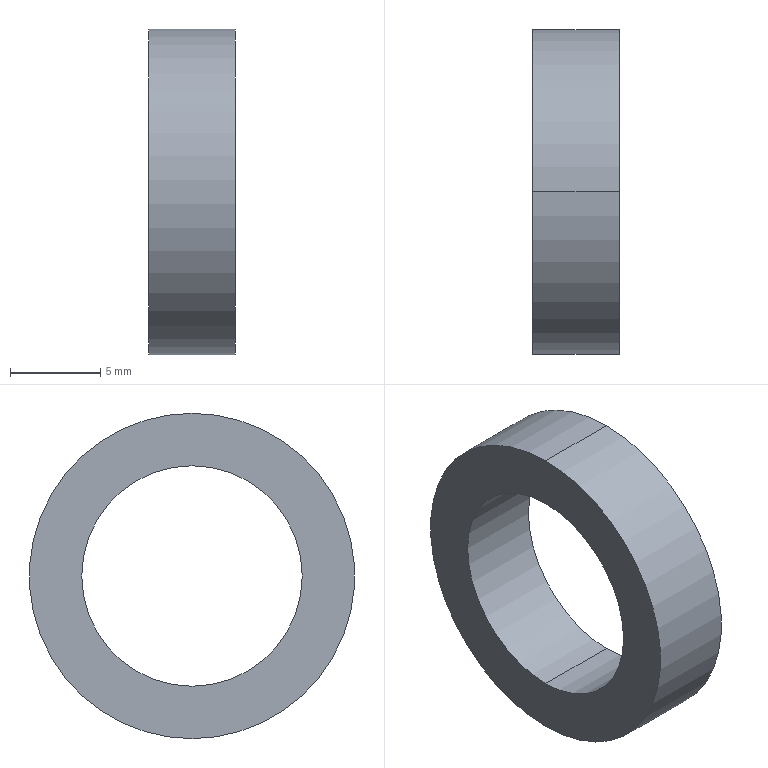Part | STEP file | Symmetry REAR WASHER BALANCER | 1 solid | 6 faces | box 4.76 x 18 x 18 mm | volume 654.835 mm3 | cylinder 4 | plane 2 | commonest cylinder face diameters 12.2 x2 18 x2
STEP:
#1=CARTESIAN_POINT('',(4.76,0.,6.1));
#2=VERTEX_POINT('',#1);
#3=CARTESIAN_POINT('',(4.76,0.,-6.1));
#4=VERTEX_POINT('',#3);
#5=CARTESIAN_POINT('',(4.76,0.,0.));
#6=DIRECTION('',(-1.,0.,0.));
#7=DIRECTION('',(0.,0.,1.));
#8=AXIS2_PLACEMENT_3D('',#5,#6,#7);
#9=CIRCLE('',#8,6.1);
#10=EDGE_CURVE('',#2,#4,#9,.T.);
#11=ORIENTED_EDGE('',*,*,#10,.F.);
#12=CARTESIAN_POINT('',(0.,0.,6.1));
#13=VERTEX_POINT('',#12);
#14=CARTESIAN_POINT('',(4.76,0.,6.1));
#15=DIRECTION('',(-1.,0.,0.));
#16=VECTOR('',#15,1000.);
#17=LINE('',#14,#16);
#18=EDGE_CURVE('',#2,#13,#17,.T.);
#19=ORIENTED_EDGE('',*,*,#18,.T.);
#20=CARTESIAN_POINT('',(0.,0.,-6.1));
#21=VERTEX_POINT('',#20);
#22=CARTESIAN_POINT('',(0.,0.,0.));
#23=DIRECTION('',(-1.,0.,0.));
#24=DIRECTION('',(0.,0.,1.));
#25=AXIS2_PLACEMENT_3D('',#22,#23,#24);
#26=CIRCLE('',#25,6.1);
#27=EDGE_CURVE('',#13,#21,#26,.T.);
#28=ORIENTED_EDGE('',*,*,#27,.T.);
#29=CARTESIAN_POINT('',(4.76,0.,-6.1));
#30=DIRECTION('',(-1.,0.,0.));
#31=VECTOR('',#30,1000.);
#32=LINE('',#29,#31);
#33=EDGE_CURVE('',#4,#21,#32,.T.);
#34=ORIENTED_EDGE('',*,*,#33,.F.);
#35=EDGE_LOOP('',(#11,#19,#28,#34));
#36=FACE_OUTER_BOUND('',#35,.T.);
#37=CARTESIAN_POINT('',(4.76,0.,0.));
#38=DIRECTION('',(-1.,0.,0.));
#39=DIRECTION('',(0.,0.,-1.));
#40=AXIS2_PLACEMENT_3D('',#37,#38,#39);
#41=CYLINDRICAL_SURFACE('',#40,6.1);
#42=ADVANCED_FACE('',(#36),#41,.F.);
#43=CARTESIAN_POINT('',(4.76,0.,-9.));
#44=VERTEX_POINT('',#43);
#45=CARTESIAN_POINT('',(4.76,0.,9.));
#46=VERTEX_POINT('',#45);
#47=CARTESIAN_POINT('',(4.76,0.,0.));
#48=DIRECTION('',(-1.,0.,0.));
#49=DIRECTION('',(0.,0.,1.));
#50=AXIS2_PLACEMENT_3D('',#47,#48,#49);
#51=CIRCLE('',#50,9.);
#52=EDGE_CURVE('',#44,#46,#51,.T.);
#53=ORIENTED_EDGE('',*,*,#52,.T.);
#54=CARTESIAN_POINT('',(0.,0.,9.));
#55=VERTEX_POINT('',#54);
#56=CARTESIAN_POINT('',(4.76,0.,9.));
#57=DIRECTION('',(-1.,0.,0.));
#58=VECTOR('',#57,1000.);
#59=LINE('',#56,#58);
#60=EDGE_CURVE('',#46,#55,#59,.T.);
#61=ORIENTED_EDGE('',*,*,#60,.T.);
#62=CARTESIAN_POINT('',(0.,0.,-9.));
#63=VERTEX_POINT('',#62);
#64=CARTESIAN_POINT('',(0.,0.,0.));
#65=DIRECTION('',(-1.,0.,0.));
#66=DIRECTION('',(0.,0.,1.));
#67=AXIS2_PLACEMENT_3D('',#64,#65,#66);
#68=CIRCLE('',#67,9.);
#69=EDGE_CURVE('',#63,#55,#68,.T.);
#70=ORIENTED_EDGE('',*,*,#69,.F.);
#71=CARTESIAN_POINT('',(4.76,0.,-9.));
#72=DIRECTION('',(-1.,0.,0.));
#73=VECTOR('',#72,1000.);
#74=LINE('',#71,#73);
#75=EDGE_CURVE('',#44,#63,#74,.T.);
#76=ORIENTED_EDGE('',*,*,#75,.F.);
#77=EDGE_LOOP('',(#53,#61,#70,#76));
#78=FACE_OUTER_BOUND('',#77,.T.);
#79=CARTESIAN_POINT('',(4.76,0.,0.));
#80=DIRECTION('',(-1.,0.,0.));
#81=DIRECTION('',(0.,0.,-1.));
#82=AXIS2_PLACEMENT_3D('',#79,#80,#81);
#83=CYLINDRICAL_SURFACE('',#82,9.);
#84=ADVANCED_FACE('',(#78),#83,.T.);
#85=ORIENTED_EDGE('',*,*,#52,.F.);
#86=CARTESIAN_POINT('',(4.76,0.,0.));
#87=DIRECTION('',(-1.,0.,0.));
#88=DIRECTION('',(0.,0.,1.));
#89=AXIS2_PLACEMENT_3D('',#86,#87,#88);
#90=CIRCLE('',#89,9.);
#91=EDGE_CURVE('',#46,#44,#90,.T.);
#92=ORIENTED_EDGE('',*,*,#91,.F.);
#93=EDGE_LOOP('',(#85,#92));
#94=FACE_OUTER_BOUND('',#93,.T.);
#95=CARTESIAN_POINT('',(4.76,0.,0.));
#96=DIRECTION('',(-1.,0.,0.));
#97=DIRECTION('',(0.,0.,1.));
#98=AXIS2_PLACEMENT_3D('',#95,#96,#97);
#99=CIRCLE('',#98,6.1);
#100=EDGE_CURVE('',#4,#2,#99,.T.);
#101=ORIENTED_EDGE('',*,*,#100,.T.);
#102=ORIENTED_EDGE('',*,*,#10,.T.);
#103=EDGE_LOOP('',(#101,#102));
#104=FACE_BOUND('',#103,.T.);
#105=CARTESIAN_POINT('',(4.76,0.,0.));
#106=DIRECTION('',(1.,0.,0.));
#107=DIRECTION('',(0.,0.,1.));
#108=AXIS2_PLACEMENT_3D('',#105,#106,#107);
#109=PLANE('',#108);
#110=ADVANCED_FACE('',(#94,#104),#109,.T.);
#111=ORIENTED_EDGE('',*,*,#69,.T.);
#112=CARTESIAN_POINT('',(0.,0.,0.));
#113=DIRECTION('',(-1.,0.,0.));
#114=DIRECTION('',(0.,0.,1.));
#115=AXIS2_PLACEMENT_3D('',#112,#113,#114);
#116=CIRCLE('',#115,9.);
#117=EDGE_CURVE('',#55,#63,#116,.T.);
#118=ORIENTED_EDGE('',*,*,#117,.T.);
#119=EDGE_LOOP('',(#111,#118));
#120=FACE_OUTER_BOUND('',#119,.T.);
#121=CARTESIAN_POINT('',(0.,0.,0.));
#122=DIRECTION('',(-1.,0.,0.));
#123=DIRECTION('',(0.,0.,1.));
#124=AXIS2_PLACEMENT_3D('',#121,#122,#123);
#125=CIRCLE('',#124,6.1);
#126=EDGE_CURVE('',#21,#13,#125,.T.);
#127=ORIENTED_EDGE('',*,*,#126,.F.);
#128=ORIENTED_EDGE('',*,*,#27,.F.);
#129=EDGE_LOOP('',(#127,#128));
#130=FACE_BOUND('',#129,.T.);
#131=CARTESIAN_POINT('',(0.,0.,0.));
#132=DIRECTION('',(1.,0.,0.));
#133=DIRECTION('',(0.,0.,1.));
#134=AXIS2_PLACEMENT_3D('',#131,#132,#133);
#135=PLANE('',#134);
#136=ADVANCED_FACE('',(#120,#130),#135,.F.);
#137=ORIENTED_EDGE('',*,*,#60,.F.);
#138=ORIENTED_EDGE('',*,*,#91,.T.);
#139=ORIENTED_EDGE('',*,*,#75,.T.);
#140=ORIENTED_EDGE('',*,*,#117,.F.);
#141=EDGE_LOOP('',(#137,#138,#139,#140));
#142=FACE_OUTER_BOUND('',#141,.T.);
#143=CARTESIAN_POINT('',(4.76,0.,0.));
#144=DIRECTION('',(-1.,0.,0.));
#145=DIRECTION('',(0.,0.,-1.));
#146=AXIS2_PLACEMENT_3D('',#143,#144,#145);
#147=CYLINDRICAL_SURFACE('',#146,9.);
#148=ADVANCED_FACE('',(#142),#147,.T.);
#149=ORIENTED_EDGE('',*,*,#18,.F.);
#150=ORIENTED_EDGE('',*,*,#100,.F.);
#151=ORIENTED_EDGE('',*,*,#33,.T.);
#152=ORIENTED_EDGE('',*,*,#126,.T.);
#153=EDGE_LOOP('',(#149,#150,#151,#152));
#154=FACE_OUTER_BOUND('',#153,.T.);
#155=CARTESIAN_POINT('',(4.76,0.,0.));
#156=DIRECTION('',(-1.,0.,0.));
#157=DIRECTION('',(0.,0.,-1.));
#158=AXIS2_PLACEMENT_3D('',#155,#156,#157);
#159=CYLINDRICAL_SURFACE('',#158,6.1);
#160=ADVANCED_FACE('',(#154),#159,.F.);
#161=CLOSED_SHELL('',(#42,#84,#110,#136,#148,#160));
#162=MANIFOLD_SOLID_BREP('',#161);
#163=CARTESIAN_POINT('',(0.,0.,0.));
#164=DIRECTION('',(0.,0.,1.));
#165=DIRECTION('',(1.,0.,0.));
#166=AXIS2_PLACEMENT_3D('',#163,#164,#165);
#167=(LENGTH_UNIT()NAMED_UNIT(*)SI_UNIT(.MILLI.,.METRE.));
#168=UNCERTAINTY_MEASURE_WITH_UNIT(LENGTH_MEASURE(0.00001),#167,'','');
#169=(NAMED_UNIT(*)PLANE_ANGLE_UNIT()SI_UNIT($,.RADIAN.));
#170=(NAMED_UNIT(*)SI_UNIT($,.STERADIAN.)SOLID_ANGLE_UNIT());
#171=(GEOMETRIC_REPRESENTATION_CONTEXT(3)GLOBAL_UNCERTAINTY_ASSIGNED_CONTEXT((#168))GLOBAL_UNIT_ASSIGNED_CONTEXT((#167,#169,#170))REPRESENTATION_CONTEXT('',''));
#172=ADVANCED_BREP_SHAPE_REPRESENTATION('',(#162,#166),#171);